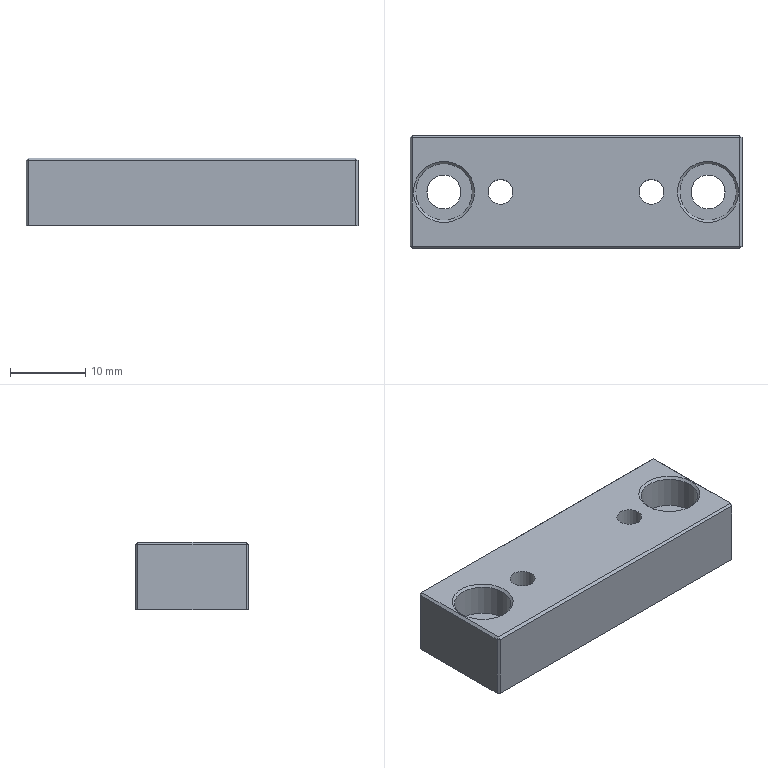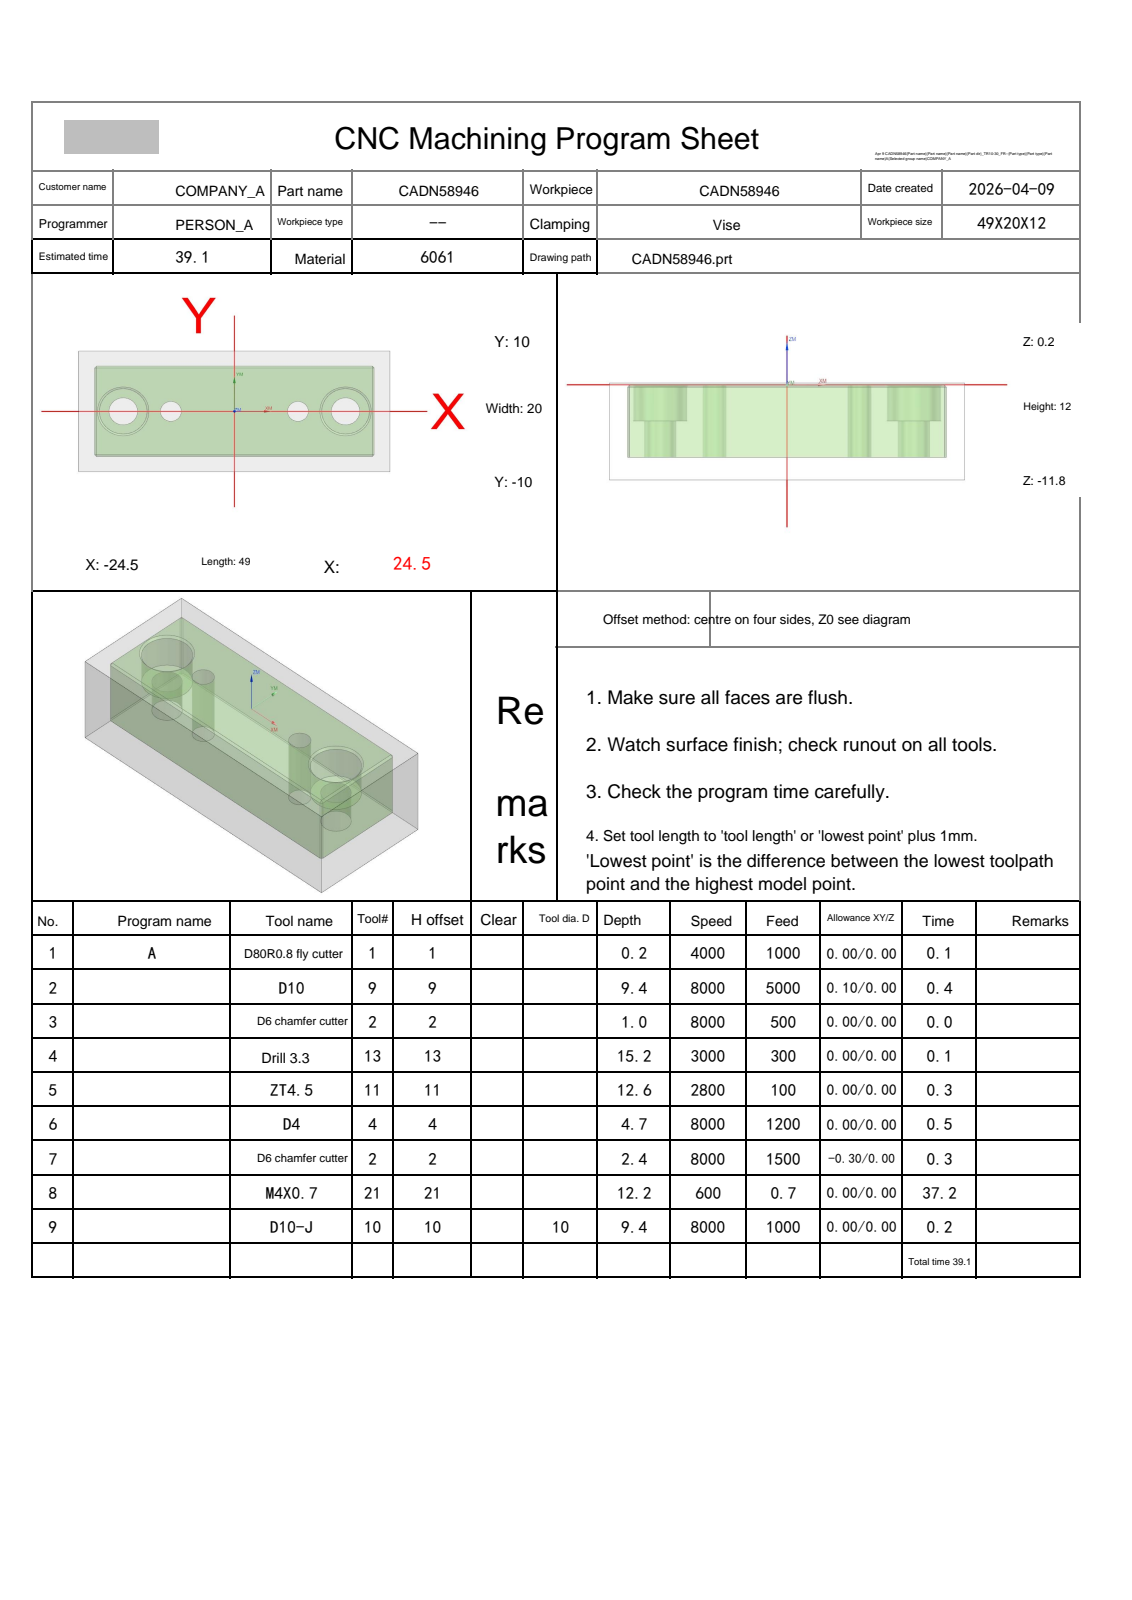NC program | NX | posted by the shop | part box 44 x 15 x 9 mm
Whole program:
%
O0001
(Machine time: 75.09 MIN)
(===Total Tool:8===)
(T1=D80R0.8 fly cutter D=80.  R=0.8  D-  H01 Z=0.    )
(T9=D10     D=10.  R=0.   D-  H09 Z=-9.2  )
(T2=D6 chamfer cutter   D=6.   R=0.   D-  H02 Z=-2.2  )
(T13=drill 3.3  D=3.3  DR_a=118 D-  H13 Z=-14.99)
(T11=ZT4.5  D=4.5  DR_a=118 D-  H11 Z=-12.35)
(T4=D4      D=4.   R=0.   D4  H04 Z=-4.5  )
(T21=M4X0.7 D=3.3  DR_a=180 D-  H21 Z=-12.  )
(T10=D10-J  D=10.  R=0.   D10 H10 Z=-9.2  )
G80 G90 G17 G49 G40
G91 G28 Z0
M01
N1 T01 M06
(D80R0.8 fly cutter  D=80. R=0.8 H=01 ce=0.00 di=0.00)
G00 G90 G54 X-67. Y0.0 M03 S4000
G43 H01 Z20.
M08
Z2.
G01 Z0.0 F1000.
X-62.
X62.
X67.
Z2.
G00 Z20.
G91 G28 Z0.0
M05
M09
G91 G28 Z0.0
M01
N2 T09 M06
(D10  D=10. R=0. H=09 ce=0.10 di=0.00)
G00 G90 G54 X0.0 Y12.6 M03 S8000
G43 H09 Z20.
M08
Z.5
G01 X21.7 Z.392 F5000.
G02 X25.306 Y11.106 Z.372 I0.0 J-5.1
G01 X25.606 Y10.806 Z.369
G02 X27.1 Y7.2 Z.349 I-3.606 J-3.606
G01 Y-7.2 Z.277
G02 X25.606 Y-10.806 Z.257 I-5.1 J0.0
G01 X25.306 Y-11.106 Z.255
G02 X21.7 Y-12.6 Z.235 I-3.606 J3.606
G01 X-21.7 Z.019
G02 X-25.306 Y-11.106 Z-.002 I0.0 J5.1
G01 X-25.606 Y-10.806 Z-.004
G02 X-27.1 Y-7.2 Z-.024 I3.606 J3.606
G01 Y7.2 Z-.096
G02 X-25.606 Y10.806 Z-.116 I5.1 J0.0
G01 X-25.306 Y11.106 Z-.118
G02 X-21.7 Y12.6 Z-.138 I3.606 J-3.606
G01 X21.7 Z-.355
G02 X25.306 Y11.106 Z-.375 I0.0 J-5.1
G01 X25.606 Y10.806 Z-.377
G02 X27.1 Y7.2 Z-.397 I-3.606 J-3.606
G01 Y-7.2 Z-.469
G02 X25.606 Y-10.806 Z-.489 I-5.1 J0.0
G01 X25.306 Y-11.106 Z-.491
G02 X21.7 Y-12.6 Z-.511 I-3.606 J3.606
G01 X-21.7 Z-.728
G02 X-25.306 Y-11.106 Z-.748 I0.0 J5.1
G01 X-25.606 Y-10.806 Z-.75
G02 X-27.1 Y-7.2 Z-.77 I3.606 J3.606
G01 Y7.2 Z-.842
G02 X-25.606 Y10.806 Z-.862 I5.1 J0.0
G01 X-25.306 Y11.106 Z-.864
G02 X-21.7 Y12.6 Z-.884 I3.606 J-3.606
G01 X21.7 Z-1.101
G02 X25.306 Y11.106 Z-1.121 I0.0 J-5.1
G01 X25.606 Y10.806 Z-1.123
G02 X27.1 Y7.2 Z-1.143 I-3.606 J-3.606
G01 Y-7.2 Z-1.215
G02 X25.606 Y-10.806 Z-1.235 I-5.1 J0.0
G01 X25.306 Y-11.106 Z-1.237
G02 X21.7 Y-12.6 Z-1.257 I-3.606 J3.606
G01 X-21.7 Z-1.474
G02 X-25.306 Y-11.106 Z-1.494 I0.0 J5.1
G01 X-25.606 Y-10.806 Z-1.496
G02 X-27.1 Y-7.2 Z-1.516 I3.606 J3.606
G01 Y7.2 Z-1.588
G02 X-25.606 Y10.806 Z-1.608 I5.1 J0.0
G01 X-25.306 Y11.106 Z-1.61
G02 X-21.7 Y12.6 Z-1.63 I3.606 J-3.606
G01 X21.7 Z-1.847
G02 X25.306 Y11.106 Z-1.867 I0.0 J-5.1
G01 X25.606 Y10.806 Z-1.869
G02 X27.1 Y7.2 Z-1.889 I-3.606 J-3.606
G01 Y-7.2 Z-1.961
G02 X25.606 Y-10.806 Z-1.981 I-5.1 J0.0
G01 X25.306 Y-11.106 Z-1.983
G02 X21.7 Y-12.6 Z-2.003 I-3.606 J3.606
G01 X-21.7 Z-2.22
G02 X-25.306 Y-11.106 Z-2.24 I0.0 J5.1
G01 X-25.606 Y-10.806 Z-2.242
G02 X-27.1 Y-7.2 Z-2.262 I3.606 J3.606
G01 Y7.2 Z-2.334
G02 X-25.606 Y10.806 Z-2.354 I5.1 J0.0
G01 X-25.306 Y11.106 Z-2.356
G02 X-21.7 Y12.6 Z-2.376 I3.606 J-3.606
G01 X21.7 Z-2.593
G02 X25.306 Y11.106 Z-2.613 I0.0 J-5.1
G01 X25.606 Y10.806 Z-2.615
G02 X27.1 Y7.2 Z-2.635 I-3.606 J-3.606
G01 Y-7.2 Z-2.707
G02 X25.606 Y-10.806 Z-2.727 I-5.1 J0.0
G01 X25.306 Y-11.106 Z-2.729
G02 X21.7 Y-12.6 Z-2.749 I-3.606 J3.606
G01 X-21.7 Z-2.966
G02 X-25.306 Y-11.106 Z-2.986 I0.0 J5.1
G01 X-25.606 Y-10.806 Z-2.988
G02 X-27.1 Y-7.2 Z-3.008 I3.606 J3.606
G01 Y7.2 Z-3.08
G02 X-25.606 Y10.806 Z-3.1 I5.1 J0.0
G01 X-25.306 Y11.106 Z-3.102
G02 X-21.7 Y12.6 Z-3.122 I3.606 J-3.606
G01 X21.7 Z-3.339
G02 X25.306 Y11.106 Z-3.359 I0.0 J-5.1
G01 X25.606 Y10.806 Z-3.361
G02 X27.1 Y7.2 Z-3.381 I-3.606 J-3.606
G01 Y-7.2 Z-3.453
G02 X25.606 Y-10.806 Z-3.473 I-5.1 J0.0
G01 X25.306 Y-11.106 Z-3.475
G02 X21.7 Y-12.6 Z-3.495 I-3.606 J3.606
G01 X-21.7 Z-3.712
G02 X-25.306 Y-11.106 Z-3.732 I0.0 J5.1
G01 X-25.606 Y-10.806 Z-3.734
G02 X-27.1 Y-7.2 Z-3.754 I3.606 J3.606
G01 Y7.2 Z-3.826
G02 X-25.606 Y10.806 Z-3.846 I5.1 J0.0
G01 X-25.306 Y11.106 Z-3.848
G02 X-21.7 Y12.6 Z-3.869 I3.606 J-3.606
G01 X21.7 Z-4.085
G02 X25.306 Y11.106 Z-4.105 I0.0 J-5.1
G01 X25.606 Y10.806 Z-4.107
G02 X27.1 Y7.2 Z-4.127 I-3.606 J-3.606
G01 Y-7.2 Z-4.199
G02 X25.606 Y-10.806 Z-4.219 I-5.1 J0.0
G01 X25.306 Y-11.106 Z-4.222
G02 X21.7 Y-12.6 Z-4.242 I-3.606 J3.606
G01 X-21.7 Z-4.458
G02 X-25.306 Y-11.106 Z-4.478 I0.0 J5.1
G01 X-25.606 Y-10.806 Z-4.481
G02 X-27.1 Y-7.2 Z-4.501 I3.606 J3.606
G01 Y7.2 Z-4.573
G02 X-25.606 Y10.806 Z-4.593 I5.1 J0.0
G01 X-25.306 Y11.106 Z-4.595
G02 X-21.7 Y12.6 Z-4.615 I3.606 J-3.606
G01 X21.7 Z-4.831
G02 X25.306 Y11.106 Z-4.852 I0.0 J-5.1
G01 X25.606 Y10.806 Z-4.854
G02 X27.1 Y7.2 Z-4.874 I-3.606 J-3.606
G01 Y-7.2 Z-4.946
G02 X25.606 Y-10.806 Z-4.966 I-5.1 J0.0
G01 X25.306 Y-11.106 Z-4.968
G02 X21.7 Y-12.6 Z-4.988 I-3.606 J3.606
G01 X-21.7 Z-5.205
G02 X-25.306 Y-11.106 Z-5.225 I0.0 J5.1
G01 X-25.606 Y-10.806 Z-5.227
G02 X-27.1 Y-7.2 Z-5.247 I3.606 J3.606
G01 Y7.2 Z-5.319
G02 X-25.606 Y10.806 Z-5.339 I5.1 J0.0
G01 X-25.306 Y11.106 Z-5.341
G02 X-21.7 Y12.6 Z-5.361 I3.606 J-3.606
G01 X21.7 Z-5.578
G02 X25.306 Y11.106 Z-5.598 I0.0 J-5.1
G01 X25.606 Y10.806 Z-5.6
G02 X27.1 Y7.2 Z-5.62 I-3.606 J-3.606
G01 Y-7.2 Z-5.692
G02 X25.606 Y-10.806 Z-5.712 I-5.1 J0.0
G01 X25.306 Y-11.106 Z-5.714
G02 X21.7 Y-12.6 Z-5.734 I-3.606 J3.606
G01 X-21.7 Z-5.951
G02 X-25.306 Y-11.106 Z-5.971 I0.0 J5.1
G01 X-25.606 Y-10.806 Z-5.973
G02 X-27.1 Y-7.2 Z-5.993 I3.606 J3.606
G01 Y7.2 Z-6.065
G02 X-25.606 Y10.806 Z-6.085 I5.1 J0.0
G01 X-25.306 Y11.106 Z-6.087
G02 X-21.7 Y12.6 Z-6.107 I3.606 J-3.606
G01 X21.7 Z-6.324
G02 X25.306 Y11.106 Z-6.344 I0.0 J-5.1
G01 X25.606 Y10.806 Z-6.346
G02 X27.1 Y7.2 Z-6.366 I-3.606 J-3.606
G01 Y-7.2 Z-6.438
G02 X25.606 Y-10.806 Z-6.458 I-5.1 J0.0
G01 X25.306 Y-11.106 Z-6.46
G02 X21.7 Y-12.6 Z-6.48 I-3.606 J3.606
G01 X-21.7 Z-6.697
G02 X-25.306 Y-11.106 Z-6.717 I0.0 J5.1
G01 X-25.606 Y-10.806 Z-6.719
G02 X-27.1 Y-7.2 Z-6.739 I3.606 J3.606
G01 Y7.2 Z-6.811
G02 X-25.606 Y10.806 Z-6.831 I5.1 J0.0
G01 X-25.306 Y11.106 Z-6.833
G02 X-21.7 Y12.6 Z-6.853 I3.606 J-3.606
G01 X21.7 Z-7.07
G02 X25.306 Y11.106 Z-7.09 I0.0 J-5.1
G01 X25.606 Y10.806 Z-7.092
G02 X27.1 Y7.2 Z-7.112 I-3.606 J-3.606
G01 Y-7.2 Z-7.184
G02 X25.606 Y-10.806 Z-7.204 I-5.1 J0.0
G01 X25.306 Y-11.106 Z-7.206
G02 X21.7 Y-12.6 Z-7.226 I-3.606 J3.606
G01 X-21.7 Z-7.443
G02 X-25.306 Y-11.106 Z-7.463 I0.0 J5.1
G01 X-25.606 Y-10.806 Z-7.465
G02 X-27.1 Y-7.2 Z-7.485 I3.606 J3.606
G01 Y7.2 Z-7.557
G02 X-25.606 Y10.806 Z-7.577 I5.1 J0.0
G01 X-25.306 Y11.106 Z-7.579
G02 X-21.7 Y12.6 Z-7.599 I3.606 J-3.606
G01 X21.7 Z-7.816
G02 X25.306 Y11.106 Z-7.836 I0.0 J-5.1
G01 X25.606 Y10.806 Z-7.838
G02 X27.1 Y7.2 Z-7.858 I-3.606 J-3.606
G01 Y-7.2 Z-7.93
G02 X25.606 Y-10.806 Z-7.95 I-5.1 J0.0
G01 X25.306 Y-11.106 Z-7.952
G02 X21.7 Y-12.6 Z-7.972 I-3.606 J3.606
G01 X-21.7 Z-8.189
G02 X-25.306 Y-11.106 Z-8.209 I0.0 J5.1
G01 X-25.606 Y-10.806 Z-8.211
G02 X-27.1 Y-7.2 Z-8.231 I3.606 J3.606
G01 Y7.2 Z-8.303
G02 X-25.606 Y10.806 Z-8.323 I5.1 J0.0
G01 X-25.306 Y11.106 Z-8.325
G02 X-21.7 Y12.6 Z-8.345 I3.606 J-3.606
G01 X21.7 Z-8.562
G02 X25.306 Y11.106 Z-8.582 I0.0 J-5.1
G01 X25.606 Y10.806 Z-8.584
G02 X27.1 Y7.2 Z-8.604 I-3.606 J-3.606
G01 Y-7.2 Z-8.676
G02 X25.606 Y-10.806 Z-8.696 I-5.1 J0.0
G01 X25.306 Y-11.106 Z-8.698
G02 X21.7 Y-12.6 Z-8.719 I-3.606 J3.606
G01 X-21.7 Z-8.935
G02 X-25.306 Y-11.106 Z-8.955 I0.0 J5.1
G01 X-25.606 Y-10.806 Z-8.957
G02 X-27.1 Y-7.2 Z-8.977 I3.606 J3.606
G01 Y7.2 Z-9.049
G02 X-25.606 Y10.806 Z-9.069 I5.1 J0.0
G01 X-25.306 Y11.106 Z-9.072
G02 X-21.7 Y12.6 Z-9.092 I3.606 J-3.606
G01 X0.0 Z-9.2
X21.7
G02 X25.306 Y11.106 I0.0 J-5.1
G01 X25.606 Y10.806
G02 X27.1 Y7.2 I-3.606 J-3.606
G01 Y-7.2
G02 X25.606 Y-10.806 I-5.1 J0.0
G01 X25.306 Y-11.106
G02 X21.7 Y-12.6 I-3.606 J3.606
G01 X-21.7
G02 X-25.306 Y-11.106 I0.0 J5.1
G01 X-25.606 Y-10.806
G02 X-27.1 Y-7.2 I3.606 J3.606
G01 Y7.2
G02 X-25.606 Y10.806 I5.1 J0.0
G01 X-25.306 Y11.106
G02 X-21.7 Y12.6 I3.606 J-3.606
G01 X0.0
X.5
Z-8.2
G00 Z20.
G91 G28 Z0.0
M05
M09
G91 G28 Z0.0
M01
N3 T02 M06
(D6 chamfer cutter  D=6. R=0. H=02 ce=0.00 di=0.00)
G00 G90 G54 X17.5 Y0.0 M03 S8000
G43 H02 Z20.
M08
G98 G81 X17.5 Y0.0 Z-.8 R1. F500.
X10.
X-10.
X-17.5
G80
G00 Z20.
G91 G28 Z0.0
M05
M09
G91 G28 Z0.0
M01
N4 T13 M06
(drill 3.3 D=3.3 DR_a=118 H=13)
G00 G90 G54 X10. Y0.0 M03 S3000
G43 H13 Z20.
M08
G98 G83 X10. Y0.0 Z-14.991 R1. F300. Q2.
X-10.
G80
G00 Z20.
G91 G28 Z0.0
M05
M09
G91 G28 Z0.0
M01
N5 T11 M06
(ZT4.5 D=4.5 DR_a=118 H=11)
G00 G90 G54 X17.5 Y0.0 M03 S2800
G43 H11 Z20.
M08
G98 G83 X17.5 Y0.0 Z-12.352 R1. F100. Q2.
X-17.5
G80
G00 Z20.
G91 G28 Z0.0
M05
M09
G91 G28 Z0.0
M01
N6 T04 M06
(D4  D=4. R=0. H=04 ce=0.10 di=0.00)
G00 G90 G54 X17.5 Y0.0 M03 S8000
G43 H04 Z20.
M08
Z.8
G03 X18.325 Y-.825 I.825 J0.0 F1200.
X19.15 Y0.0 I0.0 J.825
X19.15 Y0.0 Z.5 I-1.65 J0.0
X19.15 Y0.0 Z.2 I-1.65 J0.0
X19.15 Y0.0 Z-.1 I-1.65 J0.0
X19.15 Y0.0 Z-.4 I-1.65 J0.0
X19.15 Y0.0 Z-.7 I-1.65 J0.0
X19.15 Y0.0 Z-1. I-1.65 J0.0
X19.15 Y0.0 Z-1.3 I-1.65 J0.0
X19.15 Y0.0 Z-1.6 I-1.65 J0.0
X19.15 Y0.0 Z-1.9 I-1.65 J0.0
X19.15 Y0.0 Z-2.2 I-1.65 J0.0
X19.15 Y0.0 Z-2.5 I-1.65 J0.0
X19.15 Y0.0 Z-2.8 I-1.65 J0.0
X19.15 Y0.0 Z-3.1 I-1.65 J0.0
X19.15 Y0.0 Z-3.4 I-1.65 J0.0
X19.15 Y0.0 Z-3.7 I-1.65 J0.0
X19.15 Y0.0 Z-4. I-1.65 J0.0
X19.15 Y0.0 Z-4.3 I-1.65 J0.0
X16.675 Y-1.429 Z-4.5 I-1.65 J0.0
X17.5 Y-1.65 I.825 J1.429
X19.15 Y0.0 I0.0 J1.65
X17.5 Y1.65 I-1.65 J0.0
X15.85 Y0.0 I0.0 J-1.65
X16.675 Y-1.429 I1.65 J0.0
X17.088 Y-1.539 I.412 J.714
X17.913 Y-.714 I0.0 J.825
X17.5 Y0.0 I-.825 J0.0
G00 Z20.
X-17.5
Z.8
G03 X-16.675 Y-.825 I.825 J0.0
X-15.85 Y0.0 I0.0 J.825
X-15.85 Y0.0 Z.5 I-1.65 J0.0
X-15.85 Y0.0 Z.2 I-1.65 J0.0
X-15.85 Y0.0 Z-.1 I-1.65 J0.0
X-15.85 Y0.0 Z-.4 I-1.65 J0.0
X-15.85 Y0.0 Z-.7 I-1.65 J0.0
X-15.85 Y0.0 Z-1. I-1.65 J0.0
X-15.85 Y0.0 Z-1.3 I-1.65 J0.0
X-15.85 Y0.0 Z-1.6 I-1.65 J0.0
X-15.85 Y0.0 Z-1.9 I-1.65 J0.0
X-15.85 Y0.0 Z-2.2 I-1.65 J0.0
X-15.85 Y0.0 Z-2.5 I-1.65 J0.0
X-15.85 Y0.0 Z-2.8 I-1.65 J0.0
X-15.85 Y0.0 Z-3.1 I-1.65 J0.0
X-15.85 Y0.0 Z-3.4 I-1.65 J0.0
X-15.85 Y0.0 Z-3.7 I-1.65 J0.0
X-15.85 Y0.0 Z-4. I-1.65 J0.0
X-15.85 Y0.0 Z-4.3 I-1.65 J0.0
X-18.325 Y-1.429 Z-4.5 I-1.65 J0.0
X-17.5 Y-1.65 I.825 J1.429
X-15.85 Y0.0 I0.0 J1.65
X-17.5 Y1.65 I-1.65 J0.0
X-19.15 Y0.0 I0.0 J-1.65
X-18.325 Y-1.429 I1.65 J0.0
X-17.913 Y-1.539 I.412 J.714
X-17.088 Y-.714 I0.0 J.825
X-17.5 Y0.0 I-.825 J0.0
G00 Z20.
G00 G90 X17.5 Y0.0 M03 S8000
Z20.
Z.8
G41 D04
G01 X17.545 Y-.195 F500.
G03 X18.386 Y-.864 I.841 J.195
X19.25 Y0.0 I0.0 J.864
X19.25 Y0.0 Z-4.2 I-1.75 J0.0
X19.127 Y.644 Z-4.5 I-1.75 J0.0
X17.5 Y1.75 I-1.627 J-.644
X15.75 Y0.0 I0.0 J-1.75
X17.5 Y-1.75 I1.75 J0.0
X19.25 Y0.0 I0.0 J1.75
X19.127 Y.644 I-1.75 J0.0
X18.324 Y1.19 I-.803 J-.318
X17.461 Y.326 I0.0 J-.864
G01 X17.47 Y.198
G40 X17.5 Y0.0
G00 Z20.
X-17.5
Z.8
G41 D04
G01 X-17.455 Y-.195
G03 X-16.614 Y-.864 I.841 J.195
X-15.75 Y0.0 I0.0 J.864
X-15.75 Y0.0 Z-4.2 I-1.75 J0.0
X-15.873 Y.644 Z-4.5 I-1.75 J0.0
X-17.5 Y1.75 I-1.627 J-.644
X-19.25 Y0.0 I0.0 J-1.75
X-17.5 Y-1.75 I1.75 J0.0
X-15.75 Y0.0 I0.0 J1.75
X-15.873 Y.644 I-1.75 J0.0
X-16.676 Y1.19 I-.803 J-.318
X-17.539 Y.326 I0.0 J-.864
G01 X-17.53 Y.198
G40 X-17.5 Y0.0
G00 Z20.
G91 G28 Z0.0
M05
M09
G91 G28 Z0.0
M01
N7 T02 M06
(D6 chamfer cutter  D=6. R=0. H=02 ce=0.00 di=0.00)
G00 G90 G54 X10. Y0.0 M03 S8000
G43 H02 Z20.
M08
G98 G81 X10. Y0.0 Z-2.2 R3. F500.
X-10.
G80
G00 Z20.
G00 G90 X15.317 Y1.671 M03 S8000
Z20.
Z2.5
G01 X15.268 Y1.611 Z2.472 F500.
X15.084 Y1.32 Z2.347
X14.939 Y1.009 Z2.222
X14.833 Y.681 Z2.096
X14.769 Y.343 Z1.971
X14.747 Y0.0 Z1.846
X14.769 Y-.343 Z1.721
X14.833 Y-.681 Z1.595
X14.939 Y-1.009 Z1.47
X15.084 Y-1.32 Z1.345
X15.268 Y-1.611 Z1.22
X15.486 Y-1.877 Z1.094
X15.736 Y-2.114 Z.969
X16.014 Y-2.317 Z.844
X16.236 Y-2.446 Z.75
X16.551 Y-2.584 Z.625
X16.881 Y-2.683 Z.5
X17.22 Y-2.739 Z.375
X17.564 Y-2.752 Z.25
X17.907 Y-2.723 Z.124
X18.244 Y-2.651 Z-.001
X18.568 Y-2.537 Z-.126
X18.877 Y-2.384 Z-.251
X19.163 Y-2.194 Z-.377
X19.424 Y-1.969 Z-.502
X19.654 Y-1.714 Z-.627
X19.851 Y-1.432 Z-.752
X20.012 Y-1.127 Z-.878
X20.133 Y-.805 Z-1.003
X20.212 Y-.471 Z-1.128
X20.25 Y-.128 Z-1.253
Y0.0 Z-1.3
G03 X17.5 Y2.75 I-2.75 J0.0
X14.75 Y0.0 I0.0 J-2.75
X17.5 Y-2.75 I2.75 J0.0
X20.25 Y0.0 I0.0 J2.75
X20.205 Y.497 I-2.75 J0.0
G01 Z1.2
G00 Z20.
X-19.683 Y1.671
Z2.5
G01 X-19.732 Y1.611 Z2.472
X-19.916 Y1.32 Z2.347
X-20.061 Y1.009 Z2.222
X-20.167 Y.681 Z2.096
X-20.231 Y.343 Z1.971
X-20.253 Y0.0 Z1.846
X-20.231 Y-.343 Z1.721
X-20.167 Y-.681 Z1.595
X-20.061 Y-1.009 Z1.47
X-19.916 Y-1.32 Z1.345
X-19.732 Y-1.611 Z1.22
X-19.514 Y-1.877 Z1.094
X-19.264 Y-2.114 Z.969
X-18.986 Y-2.317 Z.844
X-18.764 Y-2.446 Z.75
X-18.449 Y-2.584 Z.625
X-18.119 Y-2.683 Z.5
X-17.78 Y-2.739 Z.375
X-17.436 Y-2.752 Z.25
X-17.093 Y-2.723 Z.124
X-16.756 Y-2.651 Z-.001
X-16.432 Y-2.537 Z-.126
X-16.124 Y-2.384 Z-.251
X-15.837 Y-2.194 Z-.377
X-15.576 Y-1.969 Z-.502
X-15.346 Y-1.714 Z-.627
X-15.149 Y-1.432 Z-.752
X-14.988 Y-1.127 Z-.878
X-14.867 Y-.805 Z-1.003
X-14.788 Y-.471 Z-1.128
X-14.75 Y-.128 Z-1.253
Y0.0 Z-1.3
G03 X-17.5 Y2.75 I-2.75 J0.0
X-20.25 Y0.0 I0.0 J-2.75
X-17.5 Y-2.75 I2.75 J0.0
X-14.75 Y0.0 I0.0 J2.75
X-14.795 Y.497 I-2.75 J0.0
G01 Z1.2
G00 Z20.
G00 G90 X-23.9 Y9.4 M03 S6500
Z20.
Z.5
G01 Z-1. F1500.
G03 X-22.7 Y8.2 I1.2 J0.0
G01 X22.7
Y-8.2
X-22.7
Y8.2
X-22.3
G03 X-21.1 Y9.4 I0.0 J1.2
G01 Z.5
G00 Z20.
G91 G28 Z0.0
M05
M09
G91 G28 Z0.0
M01
N8 T21 M06
(M4X0.7 D=3.3 DR_a=180 H=21)
G00 G90 G54 X10. Y0.0 M03 S600
G43 H21 Z20.
M08
G95
G98 G84 X10. Y0.0 Z-12. R1. F.7 Q4.
X-10.
G80
G94
G00 Z20.
G91 G28 Z0.0
M05
M09
G91 G28 Z0.0
M01
N9 T10 M06
(D10-J  D=10. R=0. H=10 ce=0.00 di=0.00)
G00 G90 G54 X22.713 Y-13.616 M03 S8000
G43 H10 Z20.
M08
Z-8.7
G01 Z-9.2 F1000.
G41 D10
X22.697 Y-13.417
G03 X21.7 Y-12.5 I-.997 J-.083
G01 X-21.7
G02 X-25.236 Y-11.036 I0.0 J5.
G01 X-25.536 Y-10.736
G02 X-27. Y-7.2 I3.536 J3.536
G01 Y7.2
G02 X-25.536 Y10.736 I5. J0.0
G01 X-25.236 Y11.036
G02 X-21.7 Y12.5 I3.536 J-3.536
G01 X21.7
G02 X25.236 Y11.036 I0.0 J-5.
G01 X25.536 Y10.736
G02 X27. Y7.2 I-3.536 J-3.536
G01 Y-7.2
G02 X25.536 Y-10.736 I-5. J0.0
G01 X25.236 Y-11.036
G02 X21.7 Y-12.5 I-3.536 J3.536
G01 X21.2
G03 X20.2 Y-13.5 I0.0 J-1.
G01 G40 Y-13.7
Z-8.7
G00 Z20.
M05
M09
G91 G28 Z0.0
G91 G28 Y0.0
M30
%